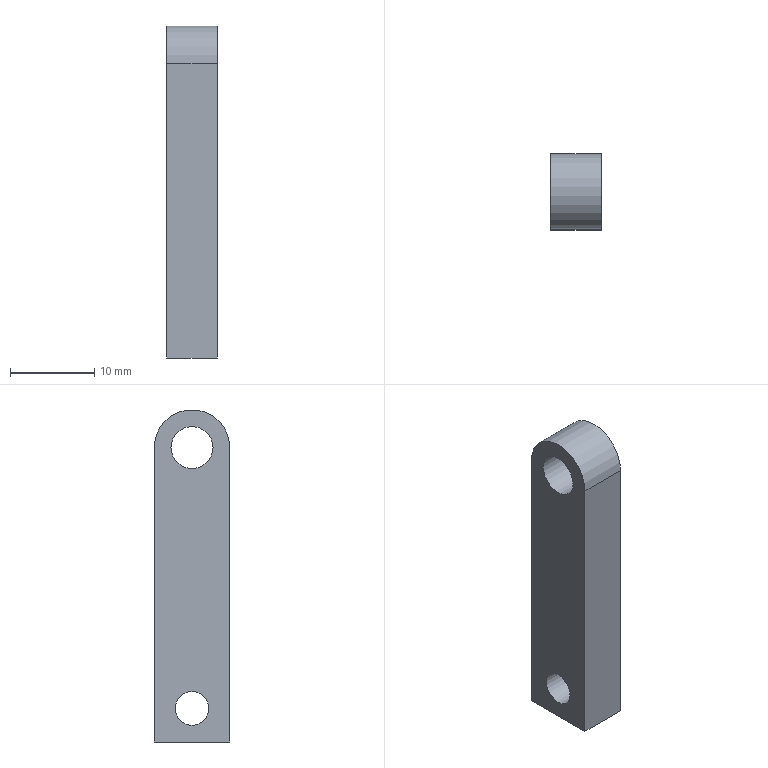Part | STEP file | 1-69.5 | 1 solid | 8 faces | box 6 x 9 x 39.5 mm | volume 1888 mm3 | plane 5 | cylinder 3 | commonest cylinder face diameters 4 x1 5 x1 9 x1
STEP:
#1=CARTESIAN_POINT('',(0.,0.,0.));
#2=DIRECTION('',(0.,0.,1.));
#3=DIRECTION('',(1.,0.,0.));
#4=AXIS2_PLACEMENT_3D('',#1,#2,#3);
#5=CARTESIAN_POINT('',(3.,4.5,0.));
#6=VERTEX_POINT('',#5);
#7=CARTESIAN_POINT('',(3.,-4.5,0.));
#8=VERTEX_POINT('',#7);
#9=CARTESIAN_POINT('',(3.,0.,0.));
#10=DIRECTION('',(1.,0.,0.));
#11=DIRECTION('',(0.,1.,0.));
#12=AXIS2_PLACEMENT_3D('',#9,#10,#11);
#13=CIRCLE('',#12,4.5);
#14=CARTESIAN_POINT('',(3.,15.25,-15.25));
#15=DIRECTION('',(1.,0.,0.));
#16=DIRECTION('',(0.,1.,0.));
#17=AXIS2_PLACEMENT_3D('',#14,#15,#16);
#18=PLANE('',#17);
#19=CARTESIAN_POINT('',(-15.25,15.25));
#20=DIRECTION('',(1.,0.));
#21=AXIS2_PLACEMENT_2D('',#19,#20);
#22=CIRCLE('',#21,4.5);
#23=(GEOMETRIC_REPRESENTATION_CONTEXT(2)PARAMETRIC_REPRESENTATION_CONTEXT()REPRESENTATION_CONTEXT('',''));
#24=DEFINITIONAL_REPRESENTATION('',(#22),#23);
#25=PCURVE('',#18,#24);
#26=CARTESIAN_POINT('',(3.,0.,0.));
#27=DIRECTION('',(-1.,0.,0.));
#28=DIRECTION('',(0.,1.,0.));
#29=AXIS2_PLACEMENT_3D('',#26,#27,#28);
#30=CYLINDRICAL_SURFACE('',#29,4.5);
#31=CARTESIAN_POINT('',(6.283,0.));
#32=DIRECTION('',(-1.,0.));
#33=VECTOR('',#32,1.);
#34=LINE('',#31,#33);
#35=(GEOMETRIC_REPRESENTATION_CONTEXT(2)PARAMETRIC_REPRESENTATION_CONTEXT()REPRESENTATION_CONTEXT('',''));
#36=DEFINITIONAL_REPRESENTATION('',(#34),#35);
#37=PCURVE('',#30,#36);
#38=SURFACE_CURVE('',#13,(#25,#37),.PCURVE_S1.);
#39=EDGE_CURVE('',#6,#8,#38,.T.);
#40=ORIENTED_EDGE('',*,*,#39,.T.);
#41=CARTESIAN_POINT('',(3.,-4.5,-35.));
#42=VERTEX_POINT('',#41);
#43=CARTESIAN_POINT('',(3.,-4.5,0.));
#44=DIRECTION('',(0.,0.,-1.));
#45=VECTOR('',#44,1.);
#46=LINE('',#43,#45);
#47=CARTESIAN_POINT('',(-19.75,15.25));
#48=DIRECTION('',(0.,-1.));
#49=VECTOR('',#48,1.);
#50=LINE('',#47,#49);
#51=(GEOMETRIC_REPRESENTATION_CONTEXT(2)PARAMETRIC_REPRESENTATION_CONTEXT()REPRESENTATION_CONTEXT('',''));
#52=DEFINITIONAL_REPRESENTATION('',(#50),#51);
#53=PCURVE('',#18,#52);
#54=CARTESIAN_POINT('',(0.,-4.5,-17.5));
#55=DIRECTION('',(0.,1.,0.));
#56=DIRECTION('',(0.,0.,-1.));
#57=AXIS2_PLACEMENT_3D('',#54,#55,#56);
#58=PLANE('',#57);
#59=CARTESIAN_POINT('',(-17.5,-3.));
#60=DIRECTION('',(1.,0.));
#61=VECTOR('',#60,1.);
#62=LINE('',#59,#61);
#63=(GEOMETRIC_REPRESENTATION_CONTEXT(2)PARAMETRIC_REPRESENTATION_CONTEXT()REPRESENTATION_CONTEXT('',''));
#64=DEFINITIONAL_REPRESENTATION('',(#62),#63);
#65=PCURVE('',#58,#64);
#66=SURFACE_CURVE('',#46,(#53,#65),.PCURVE_S1.);
#67=EDGE_CURVE('',#8,#42,#66,.T.);
#68=ORIENTED_EDGE('',*,*,#67,.T.);
#69=CARTESIAN_POINT('',(3.,4.5,-35.));
#70=VERTEX_POINT('',#69);
#71=CARTESIAN_POINT('',(3.,-4.5,-35.));
#72=DIRECTION('',(0.,1.,0.));
#73=VECTOR('',#72,1.);
#74=LINE('',#71,#73);
#75=CARTESIAN_POINT('',(-19.75,-19.75));
#76=DIRECTION('',(1.,0.));
#77=VECTOR('',#76,1.);
#78=LINE('',#75,#77);
#79=(GEOMETRIC_REPRESENTATION_CONTEXT(2)PARAMETRIC_REPRESENTATION_CONTEXT()REPRESENTATION_CONTEXT('',''));
#80=DEFINITIONAL_REPRESENTATION('',(#78),#79);
#81=PCURVE('',#18,#80);
#82=CARTESIAN_POINT('',(0.,0.,-35.));
#83=DIRECTION('',(0.,0.,1.));
#84=DIRECTION('',(0.,1.,0.));
#85=AXIS2_PLACEMENT_3D('',#82,#83,#84);
#86=PLANE('',#85);
#87=CARTESIAN_POINT('',(-4.5,-3.));
#88=DIRECTION('',(1.,0.));
#89=VECTOR('',#88,1.);
#90=LINE('',#87,#89);
#91=(GEOMETRIC_REPRESENTATION_CONTEXT(2)PARAMETRIC_REPRESENTATION_CONTEXT()REPRESENTATION_CONTEXT('',''));
#92=DEFINITIONAL_REPRESENTATION('',(#90),#91);
#93=PCURVE('',#86,#92);
#94=SURFACE_CURVE('',#74,(#81,#93),.PCURVE_S1.);
#95=EDGE_CURVE('',#42,#70,#94,.T.);
#96=ORIENTED_EDGE('',*,*,#95,.T.);
#97=CARTESIAN_POINT('',(3.,4.5,-35.));
#98=DIRECTION('',(0.,0.,1.));
#99=VECTOR('',#98,1.);
#100=LINE('',#97,#99);
#101=CARTESIAN_POINT('',(-10.75,-19.75));
#102=DIRECTION('',(0.,1.));
#103=VECTOR('',#102,1.);
#104=LINE('',#101,#103);
#105=(GEOMETRIC_REPRESENTATION_CONTEXT(2)PARAMETRIC_REPRESENTATION_CONTEXT()REPRESENTATION_CONTEXT('',''));
#106=DEFINITIONAL_REPRESENTATION('',(#104),#105);
#107=PCURVE('',#18,#106);
#108=CARTESIAN_POINT('',(0.,4.5,-17.5));
#109=DIRECTION('',(0.,-1.,0.));
#110=DIRECTION('',(0.,0.,1.));
#111=AXIS2_PLACEMENT_3D('',#108,#109,#110);
#112=PLANE('',#111);
#113=CARTESIAN_POINT('',(-17.5,-3.));
#114=DIRECTION('',(1.,0.));
#115=VECTOR('',#114,1.);
#116=LINE('',#113,#115);
#117=(GEOMETRIC_REPRESENTATION_CONTEXT(2)PARAMETRIC_REPRESENTATION_CONTEXT()REPRESENTATION_CONTEXT('',''));
#118=DEFINITIONAL_REPRESENTATION('',(#116),#117);
#119=PCURVE('',#112,#118);
#120=SURFACE_CURVE('',#100,(#107,#119),.PCURVE_S1.);
#121=EDGE_CURVE('',#70,#6,#120,.T.);
#122=ORIENTED_EDGE('',*,*,#121,.T.);
#123=EDGE_LOOP('',(#40,#68,#96,#122));
#124=FACE_BOUND('',#123,.T.);
#125=CARTESIAN_POINT('',(3.,2.5,0.));
#126=VERTEX_POINT('',#125);
#127=CARTESIAN_POINT('',(3.,0.,0.));
#128=DIRECTION('',(-1.,0.,0.));
#129=DIRECTION('',(0.,1.,0.));
#130=AXIS2_PLACEMENT_3D('',#127,#128,#129);
#131=CIRCLE('',#130,2.5);
#132=CARTESIAN_POINT('',(-12.75,15.25));
#133=CARTESIAN_POINT('',(-12.75,10.92));
#134=CARTESIAN_POINT('',(-16.5,13.085));
#135=CARTESIAN_POINT('',(-20.25,15.25));
#136=CARTESIAN_POINT('',(-16.5,17.415));
#137=CARTESIAN_POINT('',(-12.75,19.58));
#138=CARTESIAN_POINT('',(-12.75,15.25));
#139=(BOUNDED_CURVE()B_SPLINE_CURVE(2,(#132,#133,#134,#135,#136,#137,#138),.UNSPECIFIED.,.T.,.F.)B_SPLINE_CURVE_WITH_KNOTS((1,2,2,2,2,1),(-2.094,0.,2.094,4.189,6.283,8.378),.UNSPECIFIED.)CURVE()GEOMETRIC_REPRESENTATION_ITEM()RATIONAL_B_SPLINE_CURVE((1.,0.5,1.,0.5,1.,0.5,1.))REPRESENTATION_ITEM(''));
#140=(GEOMETRIC_REPRESENTATION_CONTEXT(2)PARAMETRIC_REPRESENTATION_CONTEXT()REPRESENTATION_CONTEXT('',''));
#141=DEFINITIONAL_REPRESENTATION('',(#139),#140);
#142=PCURVE('',#18,#141);
#143=CARTESIAN_POINT('',(3.,0.,0.));
#144=DIRECTION('',(-1.,0.,0.));
#145=DIRECTION('',(0.,1.,0.));
#146=AXIS2_PLACEMENT_3D('',#143,#144,#145);
#147=CYLINDRICAL_SURFACE('',#146,2.5);
#148=CARTESIAN_POINT('',(0.,0.));
#149=DIRECTION('',(1.,0.));
#150=VECTOR('',#149,1.);
#151=LINE('',#148,#150);
#152=(GEOMETRIC_REPRESENTATION_CONTEXT(2)PARAMETRIC_REPRESENTATION_CONTEXT()REPRESENTATION_CONTEXT('',''));
#153=DEFINITIONAL_REPRESENTATION('',(#151),#152);
#154=PCURVE('',#147,#153);
#155=SURFACE_CURVE('',#131,(#142,#154),.PCURVE_S1.);
#156=EDGE_CURVE('',#126,#126,#155,.T.);
#157=ORIENTED_EDGE('',*,*,#156,.T.);
#158=EDGE_LOOP('',(#157));
#159=FACE_BOUND('',#158,.T.);
#160=CARTESIAN_POINT('',(3.,2.,-31.));
#161=VERTEX_POINT('',#160);
#162=CARTESIAN_POINT('',(3.,0.,-31.));
#163=DIRECTION('',(-1.,0.,0.));
#164=DIRECTION('',(0.,1.,0.));
#165=AXIS2_PLACEMENT_3D('',#162,#163,#164);
#166=CIRCLE('',#165,2.);
#167=CARTESIAN_POINT('',(-13.25,-15.75));
#168=CARTESIAN_POINT('',(-13.25,-19.214));
#169=CARTESIAN_POINT('',(-16.25,-17.482));
#170=CARTESIAN_POINT('',(-19.25,-15.75));
#171=CARTESIAN_POINT('',(-16.25,-14.018));
#172=CARTESIAN_POINT('',(-13.25,-12.286));
#173=CARTESIAN_POINT('',(-13.25,-15.75));
#174=(BOUNDED_CURVE()B_SPLINE_CURVE(2,(#167,#168,#169,#170,#171,#172,#173),.UNSPECIFIED.,.T.,.F.)B_SPLINE_CURVE_WITH_KNOTS((1,2,2,2,2,1),(-2.094,0.,2.094,4.189,6.283,8.378),.UNSPECIFIED.)CURVE()GEOMETRIC_REPRESENTATION_ITEM()RATIONAL_B_SPLINE_CURVE((1.,0.5,1.,0.5,1.,0.5,1.))REPRESENTATION_ITEM(''));
#175=(GEOMETRIC_REPRESENTATION_CONTEXT(2)PARAMETRIC_REPRESENTATION_CONTEXT()REPRESENTATION_CONTEXT('',''));
#176=DEFINITIONAL_REPRESENTATION('',(#174),#175);
#177=PCURVE('',#18,#176);
#178=CARTESIAN_POINT('',(3.,0.,-31.));
#179=DIRECTION('',(-1.,0.,0.));
#180=DIRECTION('',(0.,1.,0.));
#181=AXIS2_PLACEMENT_3D('',#178,#179,#180);
#182=CYLINDRICAL_SURFACE('',#181,2.);
#183=CARTESIAN_POINT('',(0.,0.));
#184=DIRECTION('',(1.,0.));
#185=VECTOR('',#184,1.);
#186=LINE('',#183,#185);
#187=(GEOMETRIC_REPRESENTATION_CONTEXT(2)PARAMETRIC_REPRESENTATION_CONTEXT()REPRESENTATION_CONTEXT('',''));
#188=DEFINITIONAL_REPRESENTATION('',(#186),#187);
#189=PCURVE('',#182,#188);
#190=SURFACE_CURVE('',#166,(#177,#189),.PCURVE_S1.);
#191=EDGE_CURVE('',#161,#161,#190,.T.);
#192=ORIENTED_EDGE('',*,*,#191,.T.);
#193=EDGE_LOOP('',(#192));
#194=FACE_BOUND('',#193,.T.);
#195=ADVANCED_FACE('',(#124,#159,#194),#18,.T.);
#196=CARTESIAN_POINT('',(-3.,4.5,0.));
#197=VERTEX_POINT('',#196);
#198=CARTESIAN_POINT('',(-3.,-4.5,0.));
#199=VERTEX_POINT('',#198);
#200=CARTESIAN_POINT('',(-3.,0.,0.));
#201=DIRECTION('',(1.,0.,0.));
#202=DIRECTION('',(0.,1.,0.));
#203=AXIS2_PLACEMENT_3D('',#200,#201,#202);
#204=CIRCLE('',#203,4.5);
#205=CARTESIAN_POINT('',(-3.,15.25,-15.25));
#206=DIRECTION('',(1.,0.,0.));
#207=DIRECTION('',(0.,1.,0.));
#208=AXIS2_PLACEMENT_3D('',#205,#206,#207);
#209=PLANE('',#208);
#210=CARTESIAN_POINT('',(-15.25,15.25));
#211=DIRECTION('',(1.,0.));
#212=AXIS2_PLACEMENT_2D('',#210,#211);
#213=CIRCLE('',#212,4.5);
#214=(GEOMETRIC_REPRESENTATION_CONTEXT(2)PARAMETRIC_REPRESENTATION_CONTEXT()REPRESENTATION_CONTEXT('',''));
#215=DEFINITIONAL_REPRESENTATION('',(#213),#214);
#216=PCURVE('',#209,#215);
#217=CARTESIAN_POINT('',(6.283,6.));
#218=DIRECTION('',(-1.,0.));
#219=VECTOR('',#218,1.);
#220=LINE('',#217,#219);
#221=(GEOMETRIC_REPRESENTATION_CONTEXT(2)PARAMETRIC_REPRESENTATION_CONTEXT()REPRESENTATION_CONTEXT('',''));
#222=DEFINITIONAL_REPRESENTATION('',(#220),#221);
#223=PCURVE('',#30,#222);
#224=SURFACE_CURVE('',#204,(#216,#223),.PCURVE_S1.);
#225=EDGE_CURVE('',#197,#199,#224,.T.);
#226=ORIENTED_EDGE('',*,*,#225,.T.);
#227=CARTESIAN_POINT('',(-3.,-4.5,-35.));
#228=VERTEX_POINT('',#227);
#229=CARTESIAN_POINT('',(-3.,-4.5,0.));
#230=DIRECTION('',(0.,0.,-1.));
#231=VECTOR('',#230,1.);
#232=LINE('',#229,#231);
#233=CARTESIAN_POINT('',(-19.75,15.25));
#234=DIRECTION('',(0.,-1.));
#235=VECTOR('',#234,1.);
#236=LINE('',#233,#235);
#237=(GEOMETRIC_REPRESENTATION_CONTEXT(2)PARAMETRIC_REPRESENTATION_CONTEXT()REPRESENTATION_CONTEXT('',''));
#238=DEFINITIONAL_REPRESENTATION('',(#236),#237);
#239=PCURVE('',#209,#238);
#240=CARTESIAN_POINT('',(-17.5,3.));
#241=DIRECTION('',(1.,0.));
#242=VECTOR('',#241,1.);
#243=LINE('',#240,#242);
#244=(GEOMETRIC_REPRESENTATION_CONTEXT(2)PARAMETRIC_REPRESENTATION_CONTEXT()REPRESENTATION_CONTEXT('',''));
#245=DEFINITIONAL_REPRESENTATION('',(#243),#244);
#246=PCURVE('',#58,#245);
#247=SURFACE_CURVE('',#232,(#239,#246),.PCURVE_S1.);
#248=EDGE_CURVE('',#199,#228,#247,.T.);
#249=ORIENTED_EDGE('',*,*,#248,.T.);
#250=CARTESIAN_POINT('',(-3.,4.5,-35.));
#251=VERTEX_POINT('',#250);
#252=CARTESIAN_POINT('',(-3.,-4.5,-35.));
#253=DIRECTION('',(0.,1.,0.));
#254=VECTOR('',#253,1.);
#255=LINE('',#252,#254);
#256=CARTESIAN_POINT('',(-19.75,-19.75));
#257=DIRECTION('',(1.,0.));
#258=VECTOR('',#257,1.);
#259=LINE('',#256,#258);
#260=(GEOMETRIC_REPRESENTATION_CONTEXT(2)PARAMETRIC_REPRESENTATION_CONTEXT()REPRESENTATION_CONTEXT('',''));
#261=DEFINITIONAL_REPRESENTATION('',(#259),#260);
#262=PCURVE('',#209,#261);
#263=CARTESIAN_POINT('',(-4.5,3.));
#264=DIRECTION('',(1.,0.));
#265=VECTOR('',#264,1.);
#266=LINE('',#263,#265);
#267=(GEOMETRIC_REPRESENTATION_CONTEXT(2)PARAMETRIC_REPRESENTATION_CONTEXT()REPRESENTATION_CONTEXT('',''));
#268=DEFINITIONAL_REPRESENTATION('',(#266),#267);
#269=PCURVE('',#86,#268);
#270=SURFACE_CURVE('',#255,(#262,#269),.PCURVE_S1.);
#271=EDGE_CURVE('',#228,#251,#270,.T.);
#272=ORIENTED_EDGE('',*,*,#271,.T.);
#273=CARTESIAN_POINT('',(-3.,4.5,-35.));
#274=DIRECTION('',(0.,0.,1.));
#275=VECTOR('',#274,1.);
#276=LINE('',#273,#275);
#277=CARTESIAN_POINT('',(-10.75,-19.75));
#278=DIRECTION('',(0.,1.));
#279=VECTOR('',#278,1.);
#280=LINE('',#277,#279);
#281=(GEOMETRIC_REPRESENTATION_CONTEXT(2)PARAMETRIC_REPRESENTATION_CONTEXT()REPRESENTATION_CONTEXT('',''));
#282=DEFINITIONAL_REPRESENTATION('',(#280),#281);
#283=PCURVE('',#209,#282);
#284=CARTESIAN_POINT('',(-17.5,3.));
#285=DIRECTION('',(1.,0.));
#286=VECTOR('',#285,1.);
#287=LINE('',#284,#286);
#288=(GEOMETRIC_REPRESENTATION_CONTEXT(2)PARAMETRIC_REPRESENTATION_CONTEXT()REPRESENTATION_CONTEXT('',''));
#289=DEFINITIONAL_REPRESENTATION('',(#287),#288);
#290=PCURVE('',#112,#289);
#291=SURFACE_CURVE('',#276,(#283,#290),.PCURVE_S1.);
#292=EDGE_CURVE('',#251,#197,#291,.T.);
#293=ORIENTED_EDGE('',*,*,#292,.T.);
#294=EDGE_LOOP('',(#226,#249,#272,#293));
#295=FACE_BOUND('',#294,.F.);
#296=CARTESIAN_POINT('',(-3.,2.5,0.));
#297=VERTEX_POINT('',#296);
#298=CARTESIAN_POINT('',(-3.,0.,0.));
#299=DIRECTION('',(-1.,0.,0.));
#300=DIRECTION('',(0.,1.,0.));
#301=AXIS2_PLACEMENT_3D('',#298,#299,#300);
#302=CIRCLE('',#301,2.5);
#303=CARTESIAN_POINT('',(-12.75,15.25));
#304=CARTESIAN_POINT('',(-12.75,10.92));
#305=CARTESIAN_POINT('',(-16.5,13.085));
#306=CARTESIAN_POINT('',(-20.25,15.25));
#307=CARTESIAN_POINT('',(-16.5,17.415));
#308=CARTESIAN_POINT('',(-12.75,19.58));
#309=CARTESIAN_POINT('',(-12.75,15.25));
#310=(BOUNDED_CURVE()B_SPLINE_CURVE(2,(#303,#304,#305,#306,#307,#308,#309),.UNSPECIFIED.,.T.,.F.)B_SPLINE_CURVE_WITH_KNOTS((1,2,2,2,2,1),(-2.094,0.,2.094,4.189,6.283,8.378),.UNSPECIFIED.)CURVE()GEOMETRIC_REPRESENTATION_ITEM()RATIONAL_B_SPLINE_CURVE((1.,0.5,1.,0.5,1.,0.5,1.))REPRESENTATION_ITEM(''));
#311=(GEOMETRIC_REPRESENTATION_CONTEXT(2)PARAMETRIC_REPRESENTATION_CONTEXT()REPRESENTATION_CONTEXT('',''));
#312=DEFINITIONAL_REPRESENTATION('',(#310),#311);
#313=PCURVE('',#209,#312);
#314=CARTESIAN_POINT('',(0.,6.));
#315=DIRECTION('',(1.,0.));
#316=VECTOR('',#315,1.);
#317=LINE('',#314,#316);
#318=(GEOMETRIC_REPRESENTATION_CONTEXT(2)PARAMETRIC_REPRESENTATION_CONTEXT()REPRESENTATION_CONTEXT('',''));
#319=DEFINITIONAL_REPRESENTATION('',(#317),#318);
#320=PCURVE('',#147,#319);
#321=SURFACE_CURVE('',#302,(#313,#320),.PCURVE_S1.);
#322=EDGE_CURVE('',#297,#297,#321,.T.);
#323=ORIENTED_EDGE('',*,*,#322,.T.);
#324=EDGE_LOOP('',(#323));
#325=FACE_BOUND('',#324,.F.);
#326=CARTESIAN_POINT('',(-3.,2.,-31.));
#327=VERTEX_POINT('',#326);
#328=CARTESIAN_POINT('',(-3.,0.,-31.));
#329=DIRECTION('',(-1.,0.,0.));
#330=DIRECTION('',(0.,1.,0.));
#331=AXIS2_PLACEMENT_3D('',#328,#329,#330);
#332=CIRCLE('',#331,2.);
#333=CARTESIAN_POINT('',(-13.25,-15.75));
#334=CARTESIAN_POINT('',(-13.25,-19.214));
#335=CARTESIAN_POINT('',(-16.25,-17.482));
#336=CARTESIAN_POINT('',(-19.25,-15.75));
#337=CARTESIAN_POINT('',(-16.25,-14.018));
#338=CARTESIAN_POINT('',(-13.25,-12.286));
#339=CARTESIAN_POINT('',(-13.25,-15.75));
#340=(BOUNDED_CURVE()B_SPLINE_CURVE(2,(#333,#334,#335,#336,#337,#338,#339),.UNSPECIFIED.,.T.,.F.)B_SPLINE_CURVE_WITH_KNOTS((1,2,2,2,2,1),(-2.094,0.,2.094,4.189,6.283,8.378),.UNSPECIFIED.)CURVE()GEOMETRIC_REPRESENTATION_ITEM()RATIONAL_B_SPLINE_CURVE((1.,0.5,1.,0.5,1.,0.5,1.))REPRESENTATION_ITEM(''));
#341=(GEOMETRIC_REPRESENTATION_CONTEXT(2)PARAMETRIC_REPRESENTATION_CONTEXT()REPRESENTATION_CONTEXT('',''));
#342=DEFINITIONAL_REPRESENTATION('',(#340),#341);
#343=PCURVE('',#209,#342);
#344=CARTESIAN_POINT('',(0.,6.));
#345=DIRECTION('',(1.,0.));
#346=VECTOR('',#345,1.);
#347=LINE('',#344,#346);
#348=(GEOMETRIC_REPRESENTATION_CONTEXT(2)PARAMETRIC_REPRESENTATION_CONTEXT()REPRESENTATION_CONTEXT('',''));
#349=DEFINITIONAL_REPRESENTATION('',(#347),#348);
#350=PCURVE('',#182,#349);
#351=SURFACE_CURVE('',#332,(#343,#350),.PCURVE_S1.);
#352=EDGE_CURVE('',#327,#327,#351,.T.);
#353=ORIENTED_EDGE('',*,*,#352,.T.);
#354=EDGE_LOOP('',(#353));
#355=FACE_BOUND('',#354,.F.);
#356=ADVANCED_FACE('',(#295,#325,#355),#209,.F.);
#357=CARTESIAN_POINT('',(3.,4.5,0.));
#358=DIRECTION('',(-1.,0.,0.));
#359=VECTOR('',#358,1.);
#360=LINE('',#357,#359);
#361=CARTESIAN_POINT('',(6.283,0.));
#362=DIRECTION('',(0.,1.));
#363=VECTOR('',#362,1.);
#364=LINE('',#361,#363);
#365=(GEOMETRIC_REPRESENTATION_CONTEXT(2)PARAMETRIC_REPRESENTATION_CONTEXT()REPRESENTATION_CONTEXT('',''));
#366=DEFINITIONAL_REPRESENTATION('',(#364),#365);
#367=PCURVE('',#30,#366);
#368=CARTESIAN_POINT('',(17.5,-3.));
#369=DIRECTION('',(0.,1.));
#370=VECTOR('',#369,1.);
#371=LINE('',#368,#370);
#372=(GEOMETRIC_REPRESENTATION_CONTEXT(2)PARAMETRIC_REPRESENTATION_CONTEXT()REPRESENTATION_CONTEXT('',''));
#373=DEFINITIONAL_REPRESENTATION('',(#371),#372);
#374=PCURVE('',#112,#373);
#375=SURFACE_CURVE('',#360,(#367,#374),.PCURVE_S1.);
#376=EDGE_CURVE('',#6,#197,#375,.T.);
#377=ORIENTED_EDGE('',*,*,#376,.T.);
#378=ORIENTED_EDGE('',*,*,#225,.T.);
#379=CARTESIAN_POINT('',(3.,-4.5,0.));
#380=DIRECTION('',(-1.,0.,0.));
#381=VECTOR('',#380,1.);
#382=LINE('',#379,#381);
#383=CARTESIAN_POINT('',(3.142,0.));
#384=DIRECTION('',(0.,1.));
#385=VECTOR('',#384,1.);
#386=LINE('',#383,#385);
#387=(GEOMETRIC_REPRESENTATION_CONTEXT(2)PARAMETRIC_REPRESENTATION_CONTEXT()REPRESENTATION_CONTEXT('',''));
#388=DEFINITIONAL_REPRESENTATION('',(#386),#387);
#389=PCURVE('',#30,#388);
#390=CARTESIAN_POINT('',(-17.5,-3.));
#391=DIRECTION('',(0.,1.));
#392=VECTOR('',#391,1.);
#393=LINE('',#390,#392);
#394=(GEOMETRIC_REPRESENTATION_CONTEXT(2)PARAMETRIC_REPRESENTATION_CONTEXT()REPRESENTATION_CONTEXT('',''));
#395=DEFINITIONAL_REPRESENTATION('',(#393),#394);
#396=PCURVE('',#58,#395);
#397=SURFACE_CURVE('',#382,(#389,#396),.PCURVE_S1.);
#398=EDGE_CURVE('',#8,#199,#397,.T.);
#399=ORIENTED_EDGE('',*,*,#398,.F.);
#400=ORIENTED_EDGE('',*,*,#39,.F.);
#401=EDGE_LOOP('',(#377,#378,#399,#400));
#402=FACE_BOUND('',#401,.T.);
#403=ADVANCED_FACE('',(#402),#30,.T.);
#404=ORIENTED_EDGE('',*,*,#67,.T.);
#405=CARTESIAN_POINT('',(3.,-4.5,-35.));
#406=DIRECTION('',(-1.,0.,0.));
#407=VECTOR('',#406,1.);
#408=LINE('',#405,#407);
#409=CARTESIAN_POINT('',(17.5,-3.));
#410=DIRECTION('',(0.,1.));
#411=VECTOR('',#410,1.);
#412=LINE('',#409,#411);
#413=(GEOMETRIC_REPRESENTATION_CONTEXT(2)PARAMETRIC_REPRESENTATION_CONTEXT()REPRESENTATION_CONTEXT('',''));
#414=DEFINITIONAL_REPRESENTATION('',(#412),#413);
#415=PCURVE('',#58,#414);
#416=CARTESIAN_POINT('',(-4.5,-3.));
#417=DIRECTION('',(0.,1.));
#418=VECTOR('',#417,1.);
#419=LINE('',#416,#418);
#420=(GEOMETRIC_REPRESENTATION_CONTEXT(2)PARAMETRIC_REPRESENTATION_CONTEXT()REPRESENTATION_CONTEXT('',''));
#421=DEFINITIONAL_REPRESENTATION('',(#419),#420);
#422=PCURVE('',#86,#421);
#423=SURFACE_CURVE('',#408,(#415,#422),.PCURVE_S1.);
#424=EDGE_CURVE('',#42,#228,#423,.T.);
#425=ORIENTED_EDGE('',*,*,#424,.T.);
#426=ORIENTED_EDGE('',*,*,#248,.F.);
#427=ORIENTED_EDGE('',*,*,#398,.F.);
#428=EDGE_LOOP('',(#404,#425,#426,#427));
#429=FACE_BOUND('',#428,.F.);
#430=ADVANCED_FACE('',(#429),#58,.F.);
#431=ORIENTED_EDGE('',*,*,#95,.T.);
#432=CARTESIAN_POINT('',(3.,4.5,-35.));
#433=DIRECTION('',(-1.,0.,0.));
#434=VECTOR('',#433,1.);
#435=LINE('',#432,#434);
#436=CARTESIAN_POINT('',(4.5,-3.));
#437=DIRECTION('',(0.,1.));
#438=VECTOR('',#437,1.);
#439=LINE('',#436,#438);
#440=(GEOMETRIC_REPRESENTATION_CONTEXT(2)PARAMETRIC_REPRESENTATION_CONTEXT()REPRESENTATION_CONTEXT('',''));
#441=DEFINITIONAL_REPRESENTATION('',(#439),#440);
#442=PCURVE('',#86,#441);
#443=CARTESIAN_POINT('',(-17.5,-3.));
#444=DIRECTION('',(0.,1.));
#445=VECTOR('',#444,1.);
#446=LINE('',#443,#445);
#447=(GEOMETRIC_REPRESENTATION_CONTEXT(2)PARAMETRIC_REPRESENTATION_CONTEXT()REPRESENTATION_CONTEXT('',''));
#448=DEFINITIONAL_REPRESENTATION('',(#446),#447);
#449=PCURVE('',#112,#448);
#450=SURFACE_CURVE('',#435,(#442,#449),.PCURVE_S1.);
#451=EDGE_CURVE('',#70,#251,#450,.T.);
#452=ORIENTED_EDGE('',*,*,#451,.T.);
#453=ORIENTED_EDGE('',*,*,#271,.F.);
#454=ORIENTED_EDGE('',*,*,#424,.F.);
#455=EDGE_LOOP('',(#431,#452,#453,#454));
#456=FACE_BOUND('',#455,.F.);
#457=ADVANCED_FACE('',(#456),#86,.F.);
#458=ORIENTED_EDGE('',*,*,#121,.T.);
#459=ORIENTED_EDGE('',*,*,#376,.T.);
#460=ORIENTED_EDGE('',*,*,#292,.F.);
#461=ORIENTED_EDGE('',*,*,#451,.F.);
#462=EDGE_LOOP('',(#458,#459,#460,#461));
#463=FACE_BOUND('',#462,.F.);
#464=ADVANCED_FACE('',(#463),#112,.F.);
#465=ORIENTED_EDGE('',*,*,#156,.T.);
#466=CARTESIAN_POINT('',(3.,2.5,0.));
#467=DIRECTION('',(-1.,0.,0.));
#468=VECTOR('',#467,1.);
#469=LINE('',#466,#468);
#470=CARTESIAN_POINT('',(6.283,0.));
#471=DIRECTION('',(0.,1.));
#472=VECTOR('',#471,1.);
#473=LINE('',#470,#472);
#474=(GEOMETRIC_REPRESENTATION_CONTEXT(2)PARAMETRIC_REPRESENTATION_CONTEXT()REPRESENTATION_CONTEXT('',''));
#475=DEFINITIONAL_REPRESENTATION('',(#473),#474);
#476=PCURVE('',#147,#475);
#477=CARTESIAN_POINT('',(0.,0.));
#478=DIRECTION('',(0.,1.));
#479=VECTOR('',#478,1.);
#480=LINE('',#477,#479);
#481=(GEOMETRIC_REPRESENTATION_CONTEXT(2)PARAMETRIC_REPRESENTATION_CONTEXT()REPRESENTATION_CONTEXT('',''));
#482=DEFINITIONAL_REPRESENTATION('',(#480),#481);
#483=PCURVE('',#147,#482);
#484=SEAM_CURVE('',#469,(#476,#483),.PCURVE_S1.);
#485=EDGE_CURVE('',#126,#297,#484,.T.);
#486=ORIENTED_EDGE('',*,*,#485,.T.);
#487=ORIENTED_EDGE('',*,*,#322,.F.);
#488=ORIENTED_EDGE('',*,*,#485,.F.);
#489=EDGE_LOOP('',(#465,#486,#487,#488));
#490=FACE_BOUND('',#489,.F.);
#491=ADVANCED_FACE('',(#490),#147,.F.);
#492=ORIENTED_EDGE('',*,*,#191,.T.);
#493=CARTESIAN_POINT('',(3.,2.,-31.));
#494=DIRECTION('',(-1.,0.,0.));
#495=VECTOR('',#494,1.);
#496=LINE('',#493,#495);
#497=CARTESIAN_POINT('',(6.283,0.));
#498=DIRECTION('',(0.,1.));
#499=VECTOR('',#498,1.);
#500=LINE('',#497,#499);
#501=(GEOMETRIC_REPRESENTATION_CONTEXT(2)PARAMETRIC_REPRESENTATION_CONTEXT()REPRESENTATION_CONTEXT('',''));
#502=DEFINITIONAL_REPRESENTATION('',(#500),#501);
#503=PCURVE('',#182,#502);
#504=CARTESIAN_POINT('',(0.,0.));
#505=DIRECTION('',(0.,1.));
#506=VECTOR('',#505,1.);
#507=LINE('',#504,#506);
#508=(GEOMETRIC_REPRESENTATION_CONTEXT(2)PARAMETRIC_REPRESENTATION_CONTEXT()REPRESENTATION_CONTEXT('',''));
#509=DEFINITIONAL_REPRESENTATION('',(#507),#508);
#510=PCURVE('',#182,#509);
#511=SEAM_CURVE('',#496,(#503,#510),.PCURVE_S1.);
#512=EDGE_CURVE('',#161,#327,#511,.T.);
#513=ORIENTED_EDGE('',*,*,#512,.T.);
#514=ORIENTED_EDGE('',*,*,#352,.F.);
#515=ORIENTED_EDGE('',*,*,#512,.F.);
#516=EDGE_LOOP('',(#492,#513,#514,#515));
#517=FACE_BOUND('',#516,.F.);
#518=ADVANCED_FACE('',(#517),#182,.F.);
#519=CLOSED_SHELL('',(#195,#356,#403,#430,#457,#464,#491,#518));
#520=MANIFOLD_SOLID_BREP('',#519);
#521=(LENGTH_UNIT()NAMED_UNIT(*)SI_UNIT(.MILLI.,.METRE.));
#522=UNCERTAINTY_MEASURE_WITH_UNIT(LENGTH_MEASURE(0.0000001),#521,'','');
#523=(NAMED_UNIT(*)PLANE_ANGLE_UNIT()SI_UNIT($,.RADIAN.));
#524=(NAMED_UNIT(*)SI_UNIT($,.STERADIAN.)SOLID_ANGLE_UNIT());
#525=(GEOMETRIC_REPRESENTATION_CONTEXT(3)GLOBAL_UNCERTAINTY_ASSIGNED_CONTEXT((#522))GLOBAL_UNIT_ASSIGNED_CONTEXT((#521,#523,#524))REPRESENTATION_CONTEXT('',''));
#526=ADVANCED_BREP_SHAPE_REPRESENTATION('',(#4,#520),#525);